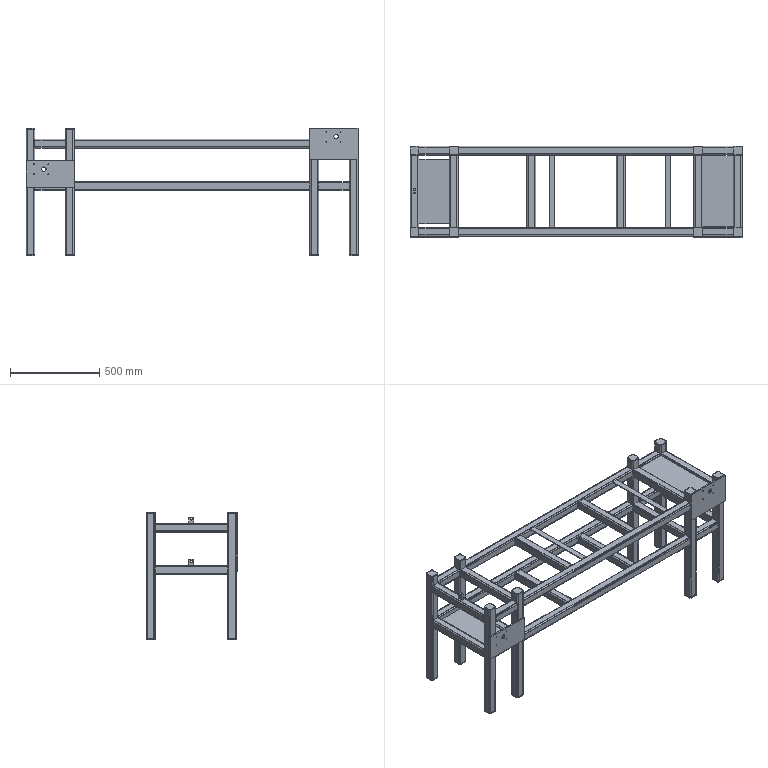Part | STEP file | MYT-A01-P01(default_machined_) | 56 solids | 828 faces | box 1860 x 514 x 715 mm | volume 13979355 mm3 | plane 528 | cylinder 300 | commonest cylinder face diameters 8 x128 16 x128 4.2 x16 14 x16 13 x4 20 x4